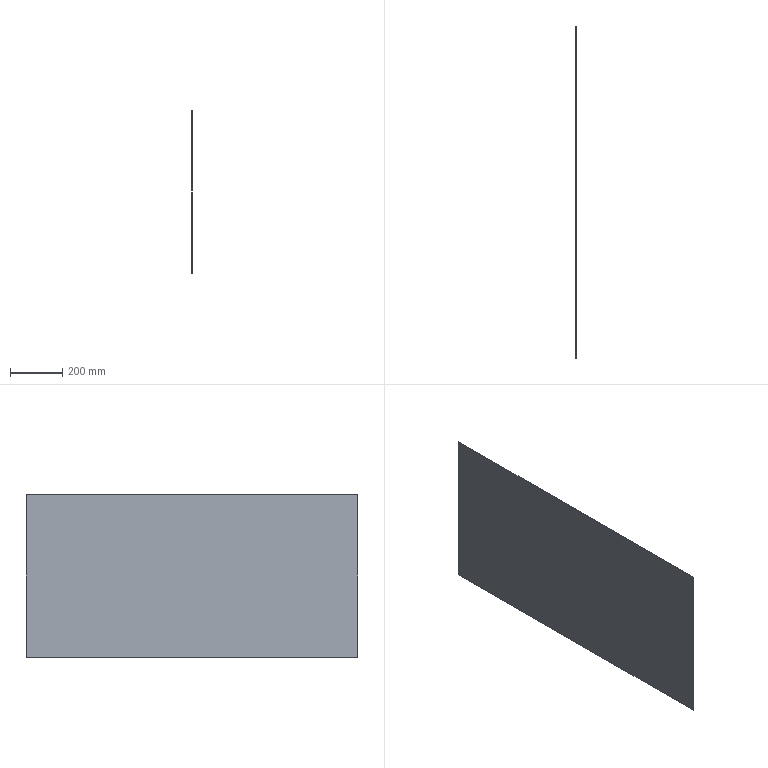Part | SolidWorks | 1 solid | 6 faces | box 1.5 x 1265 x 620 mm | volume 1176450 mm3 | plane 6
STEP:
#1=CARTESIAN_POINT('',(0.,632.5,310.));
#2=VERTEX_POINT('',#1);
#3=CARTESIAN_POINT('',(0.,-632.5,310.));
#4=VERTEX_POINT('',#3);
#5=CARTESIAN_POINT('',(0.,-632.5,310.));
#6=DIRECTION('',(0.,-1.,0.));
#7=VECTOR('',#6,1000.);
#8=LINE('',#5,#7);
#9=EDGE_CURVE('',#2,#4,#8,.T.);
#10=ORIENTED_EDGE('',*,*,#9,.F.);
#11=CARTESIAN_POINT('',(-1.5,632.5,310.));
#12=VERTEX_POINT('',#11);
#13=CARTESIAN_POINT('',(-1.5,632.5,310.));
#14=DIRECTION('',(1.,0.,0.));
#15=VECTOR('',#14,1000.);
#16=LINE('',#13,#15);
#17=EDGE_CURVE('',#12,#2,#16,.T.);
#18=ORIENTED_EDGE('',*,*,#17,.F.);
#19=CARTESIAN_POINT('',(-1.5,-632.5,310.));
#20=VERTEX_POINT('',#19);
#21=CARTESIAN_POINT('',(-1.5,-632.5,310.));
#22=DIRECTION('',(0.,-1.,0.));
#23=VECTOR('',#22,1000.);
#24=LINE('',#21,#23);
#25=EDGE_CURVE('',#12,#20,#24,.T.);
#26=ORIENTED_EDGE('',*,*,#25,.T.);
#27=CARTESIAN_POINT('',(-1.5,-632.5,310.));
#28=DIRECTION('',(1.,0.,0.));
#29=VECTOR('',#28,1000.);
#30=LINE('',#27,#29);
#31=EDGE_CURVE('',#20,#4,#30,.T.);
#32=ORIENTED_EDGE('',*,*,#31,.T.);
#33=EDGE_LOOP('',(#10,#18,#26,#32));
#34=FACE_OUTER_BOUND('',#33,.T.);
#35=CARTESIAN_POINT('',(-1.5,-632.5,310.));
#36=DIRECTION('',(0.,0.,1.));
#37=DIRECTION('',(1.,0.,0.));
#38=AXIS2_PLACEMENT_3D('',#35,#36,#37);
#39=PLANE('',#38);
#40=ADVANCED_FACE('',(#34),#39,.T.);
#41=CARTESIAN_POINT('',(0.,632.5,-310.));
#42=VERTEX_POINT('',#41);
#43=CARTESIAN_POINT('',(0.,632.5,-310.));
#44=DIRECTION('',(0.,0.,1.));
#45=VECTOR('',#44,1000.);
#46=LINE('',#43,#45);
#47=EDGE_CURVE('',#42,#2,#46,.T.);
#48=ORIENTED_EDGE('',*,*,#47,.F.);
#49=CARTESIAN_POINT('',(-1.5,632.5,-310.));
#50=VERTEX_POINT('',#49);
#51=CARTESIAN_POINT('',(-1.5,632.5,-310.));
#52=DIRECTION('',(1.,0.,0.));
#53=VECTOR('',#52,1000.);
#54=LINE('',#51,#53);
#55=EDGE_CURVE('',#50,#42,#54,.T.);
#56=ORIENTED_EDGE('',*,*,#55,.F.);
#57=CARTESIAN_POINT('',(-1.5,632.5,-310.));
#58=DIRECTION('',(0.,0.,1.));
#59=VECTOR('',#58,1000.);
#60=LINE('',#57,#59);
#61=EDGE_CURVE('',#50,#12,#60,.T.);
#62=ORIENTED_EDGE('',*,*,#61,.T.);
#63=ORIENTED_EDGE('',*,*,#17,.T.);
#64=EDGE_LOOP('',(#48,#56,#62,#63));
#65=FACE_OUTER_BOUND('',#64,.T.);
#66=CARTESIAN_POINT('',(-1.5,632.5,-310.));
#67=DIRECTION('',(0.,1.,0.));
#68=DIRECTION('',(0.,0.,1.));
#69=AXIS2_PLACEMENT_3D('',#66,#67,#68);
#70=PLANE('',#69);
#71=ADVANCED_FACE('',(#65),#70,.T.);
#72=CARTESIAN_POINT('',(0.,-632.5,-310.));
#73=VERTEX_POINT('',#72);
#74=CARTESIAN_POINT('',(0.,-632.5,-310.));
#75=DIRECTION('',(0.,1.,0.));
#76=VECTOR('',#75,1000.);
#77=LINE('',#74,#76);
#78=EDGE_CURVE('',#73,#42,#77,.T.);
#79=ORIENTED_EDGE('',*,*,#78,.F.);
#80=CARTESIAN_POINT('',(-1.5,-632.5,-310.));
#81=VERTEX_POINT('',#80);
#82=CARTESIAN_POINT('',(-1.5,-632.5,-310.));
#83=DIRECTION('',(1.,0.,0.));
#84=VECTOR('',#83,1000.);
#85=LINE('',#82,#84);
#86=EDGE_CURVE('',#81,#73,#85,.T.);
#87=ORIENTED_EDGE('',*,*,#86,.F.);
#88=CARTESIAN_POINT('',(-1.5,-632.5,-310.));
#89=DIRECTION('',(0.,1.,0.));
#90=VECTOR('',#89,1000.);
#91=LINE('',#88,#90);
#92=EDGE_CURVE('',#81,#50,#91,.T.);
#93=ORIENTED_EDGE('',*,*,#92,.T.);
#94=ORIENTED_EDGE('',*,*,#55,.T.);
#95=EDGE_LOOP('',(#79,#87,#93,#94));
#96=FACE_OUTER_BOUND('',#95,.T.);
#97=CARTESIAN_POINT('',(-1.5,-632.5,-310.));
#98=DIRECTION('',(0.,0.,-1.));
#99=DIRECTION('',(-1.,0.,0.));
#100=AXIS2_PLACEMENT_3D('',#97,#98,#99);
#101=PLANE('',#100);
#102=ADVANCED_FACE('',(#96),#101,.T.);
#103=CARTESIAN_POINT('',(0.,-632.5,-310.));
#104=DIRECTION('',(0.,0.,-1.));
#105=VECTOR('',#104,1000.);
#106=LINE('',#103,#105);
#107=EDGE_CURVE('',#4,#73,#106,.T.);
#108=ORIENTED_EDGE('',*,*,#107,.F.);
#109=ORIENTED_EDGE('',*,*,#31,.F.);
#110=CARTESIAN_POINT('',(-1.5,-632.5,-310.));
#111=DIRECTION('',(0.,0.,-1.));
#112=VECTOR('',#111,1000.);
#113=LINE('',#110,#112);
#114=EDGE_CURVE('',#20,#81,#113,.T.);
#115=ORIENTED_EDGE('',*,*,#114,.T.);
#116=ORIENTED_EDGE('',*,*,#86,.T.);
#117=EDGE_LOOP('',(#108,#109,#115,#116));
#118=FACE_OUTER_BOUND('',#117,.T.);
#119=CARTESIAN_POINT('',(-1.5,-632.5,-310.));
#120=DIRECTION('',(0.,-1.,0.));
#121=DIRECTION('',(0.,0.,-1.));
#122=AXIS2_PLACEMENT_3D('',#119,#120,#121);
#123=PLANE('',#122);
#124=ADVANCED_FACE('',(#118),#123,.T.);
#125=ORIENTED_EDGE('',*,*,#25,.F.);
#126=ORIENTED_EDGE('',*,*,#61,.F.);
#127=ORIENTED_EDGE('',*,*,#92,.F.);
#128=ORIENTED_EDGE('',*,*,#114,.F.);
#129=EDGE_LOOP('',(#125,#126,#127,#128));
#130=FACE_OUTER_BOUND('',#129,.T.);
#131=CARTESIAN_POINT('',(-1.5,0.,0.));
#132=DIRECTION('',(1.,0.,0.));
#133=DIRECTION('',(0.,0.,-1.));
#134=AXIS2_PLACEMENT_3D('',#131,#132,#133);
#135=PLANE('',#134);
#136=ADVANCED_FACE('',(#130),#135,.F.);
#137=ORIENTED_EDGE('',*,*,#9,.T.);
#138=ORIENTED_EDGE('',*,*,#107,.T.);
#139=ORIENTED_EDGE('',*,*,#78,.T.);
#140=ORIENTED_EDGE('',*,*,#47,.T.);
#141=EDGE_LOOP('',(#137,#138,#139,#140));
#142=FACE_OUTER_BOUND('',#141,.T.);
#143=CARTESIAN_POINT('',(0.,0.,0.));
#144=DIRECTION('',(1.,0.,0.));
#145=DIRECTION('',(0.,0.,-1.));
#146=AXIS2_PLACEMENT_3D('',#143,#144,#145);
#147=PLANE('',#146);
#148=ADVANCED_FACE('',(#142),#147,.T.);
#149=CLOSED_SHELL('',(#40,#71,#102,#124,#136,#148));
#150=MANIFOLD_SOLID_BREP('',#149);
#151=CARTESIAN_POINT('',(0.,0.,0.));
#152=DIRECTION('',(0.,0.,1.));
#153=DIRECTION('',(1.,0.,0.));
#154=AXIS2_PLACEMENT_3D('',#151,#152,#153);
#155=(LENGTH_UNIT()NAMED_UNIT(*)SI_UNIT(.MILLI.,.METRE.));
#156=UNCERTAINTY_MEASURE_WITH_UNIT(LENGTH_MEASURE(0.00001),#155,'','');
#157=(NAMED_UNIT(*)PLANE_ANGLE_UNIT()SI_UNIT($,.RADIAN.));
#158=(NAMED_UNIT(*)SI_UNIT($,.STERADIAN.)SOLID_ANGLE_UNIT());
#159=(GEOMETRIC_REPRESENTATION_CONTEXT(3)GLOBAL_UNCERTAINTY_ASSIGNED_CONTEXT((#156))GLOBAL_UNIT_ASSIGNED_CONTEXT((#155,#157,#158))REPRESENTATION_CONTEXT('',''));
#160=ADVANCED_BREP_SHAPE_REPRESENTATION('',(#150,#154),#159);